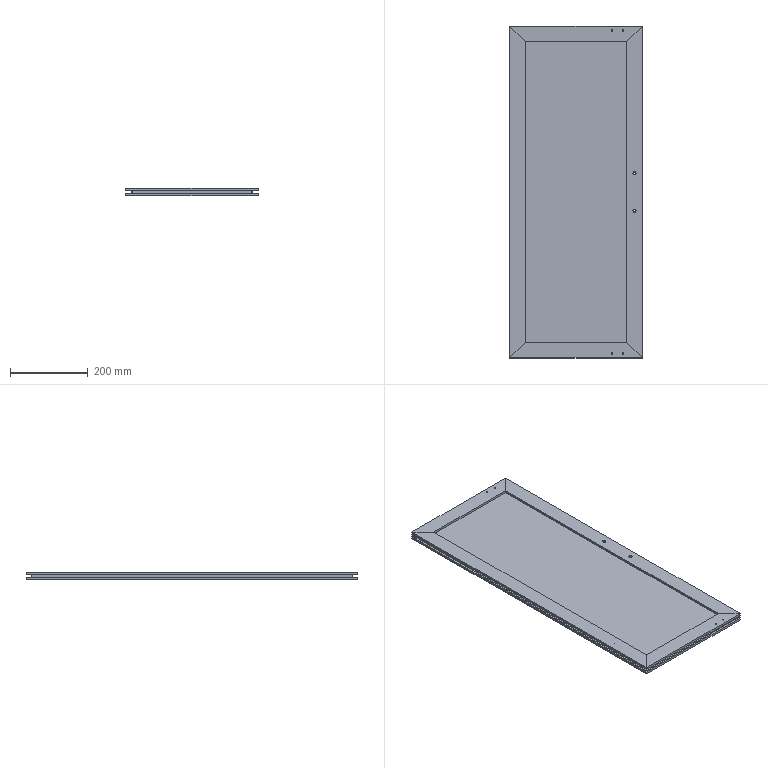Part | SolidWorks | features HoleWzd 3, ICE 1, WeldMemberFeat 1, WeldmentFeature 1 | 5 solids | 184 faces | box 341.5 x 856 x 20 mm | volume 1950280 mm3 | plane 132 | cylinder 44 | cone 8 | commonest cylinder face diameters 5 x16 3.3 x8 4.5 x8 6.5 x8 8 x4